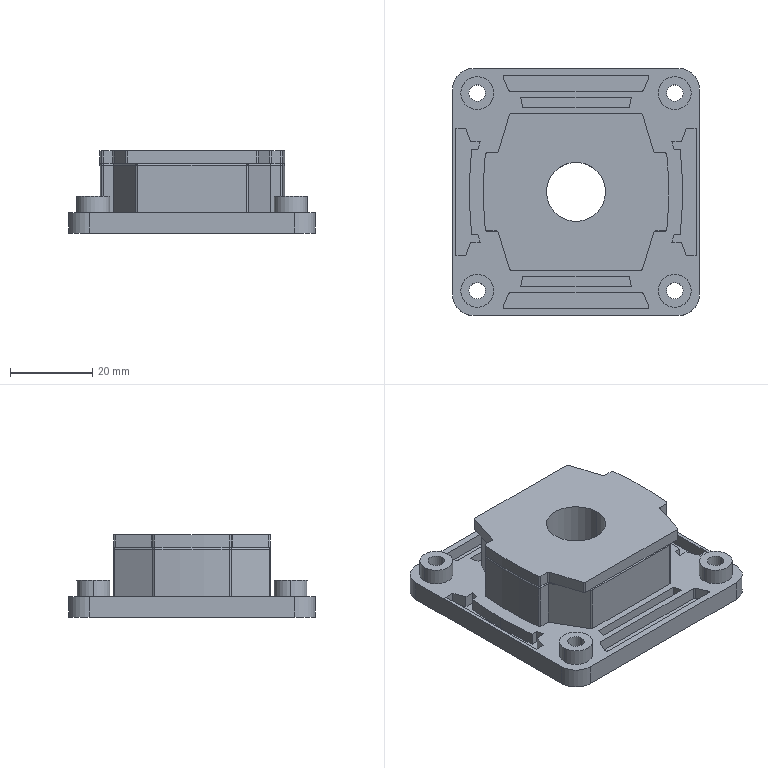Part | STEP file | PRT0120_3.stp | 1 solid | 155 faces | box 60 x 60 x 20 mm | volume 35294 mm3 | plane 76 | cylinder 69 | sphere 8 | torus 2 | commonest cylinder face diameters 1 x38 4 x8 8 x8 181 x6 10 x4 199.583 x3